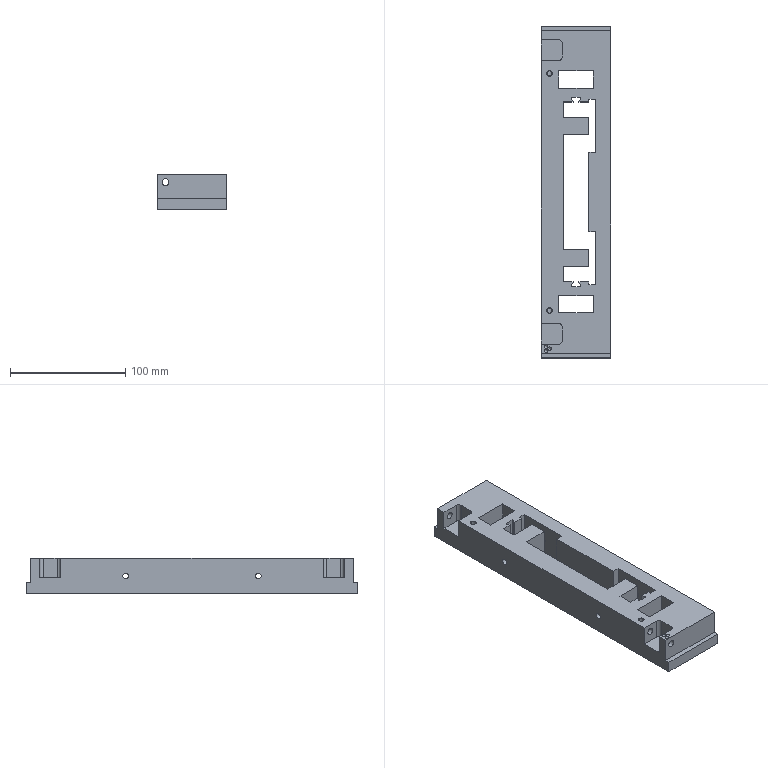Part | STEP file | 200 mesh_id2158 | 1 solid | 88 faces | box 60 x 288 x 31.2 mm | volume 373358 mm3 | plane 54 | cylinder 23 | cone 9 | spline 2 | commonest cylinder face diameters 0.52 x4 1.08 x4 5.01 x4 6 x4 6.01 x3 4.2 x2